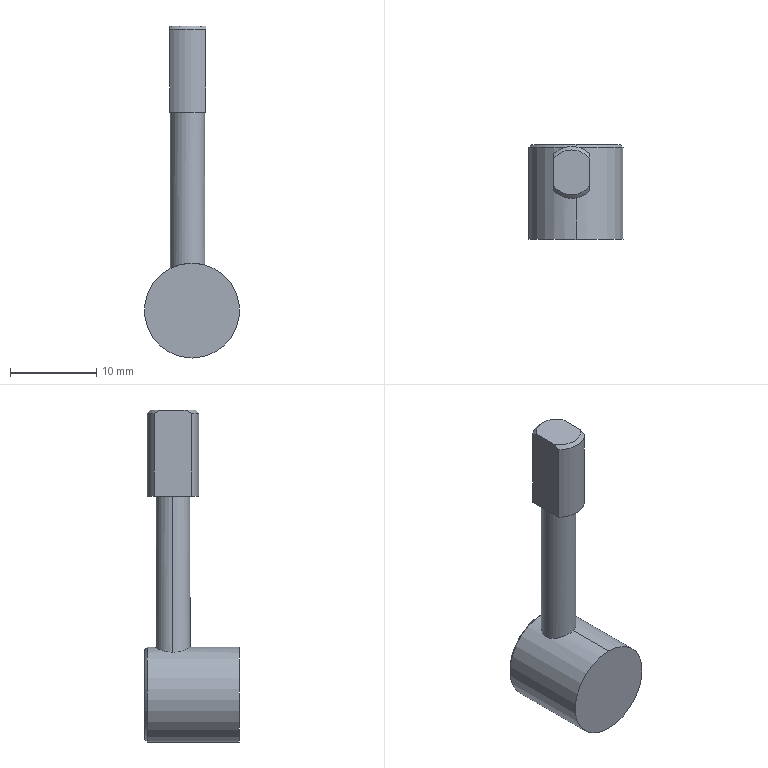Part | STEP file | l_SECWK14 | 1 solid | 23 faces | box 11 x 11 x 38.5 mm | volume 1486 mm3 | cylinder 8 | cone 8 | plane 7 | commonest cylinder face diameters 6 x4 4 x2 11 x2
STEP:
#1=CARTESIAN_POINT('',(-0.5,10.9,-3.));
#2=VERTEX_POINT('',#1);
#3=CARTESIAN_POINT('',(-0.5,10.9,3.));
#4=VERTEX_POINT('',#3);
#5=CARTESIAN_POINT('',(-0.5,10.9,0.));
#6=DIRECTION('',(0.,1.,0.));
#7=DIRECTION('',(0.,0.,1.));
#8=AXIS2_PLACEMENT_3D('',#5,#6,#7);
#9=CIRCLE('',#8,3.);
#10=EDGE_CURVE('',#2,#4,#9,.T.);
#11=ORIENTED_EDGE('',*,*,#10,.T.);
#12=CARTESIAN_POINT('',(-0.5,10.3,3.));
#13=VERTEX_POINT('',#12);
#14=CARTESIAN_POINT('',(-0.5,11.,3.));
#15=DIRECTION('',(0.,-1.,0.));
#16=VECTOR('',#15,1000.);
#17=LINE('',#14,#16);
#18=EDGE_CURVE('',#4,#13,#17,.T.);
#19=ORIENTED_EDGE('',*,*,#18,.T.);
#20=CARTESIAN_POINT('',(-0.5,10.3,-3.));
#21=VERTEX_POINT('',#20);
#22=CARTESIAN_POINT('',(-0.5,10.3,0.));
#23=DIRECTION('',(0.,1.,0.));
#24=DIRECTION('',(0.,0.,-1.));
#25=AXIS2_PLACEMENT_3D('',#22,#23,#24);
#26=CIRCLE('',#25,3.);
#27=EDGE_CURVE('',#21,#13,#26,.T.);
#28=ORIENTED_EDGE('',*,*,#27,.F.);
#29=CARTESIAN_POINT('',(-0.5,11.,-3.));
#30=DIRECTION('',(0.,-1.,0.));
#31=VECTOR('',#30,1000.);
#32=LINE('',#29,#31);
#33=EDGE_CURVE('',#2,#21,#32,.T.);
#34=ORIENTED_EDGE('',*,*,#33,.F.);
#35=EDGE_LOOP('',(#11,#19,#28,#34));
#36=FACE_OUTER_BOUND('',#35,.T.);
#37=CARTESIAN_POINT('',(-0.5,11.,0.));
#38=DIRECTION('',(0.,-1.,0.));
#39=DIRECTION('',(0.,0.,-1.));
#40=AXIS2_PLACEMENT_3D('',#37,#38,#39);
#41=CYLINDRICAL_SURFACE('',#40,3.);
#42=ADVANCED_FACE('',(#36),#41,.F.);
#43=CARTESIAN_POINT('',(-0.5,10.8,2.5));
#44=VERTEX_POINT('',#43);
#45=CARTESIAN_POINT('',(-0.5,10.8,-2.5));
#46=VERTEX_POINT('',#45);
#47=CARTESIAN_POINT('',(-0.5,10.8,0.));
#48=DIRECTION('',(0.,1.,0.));
#49=DIRECTION('',(0.,0.,1.));
#50=AXIS2_PLACEMENT_3D('',#47,#48,#49);
#51=CIRCLE('',#50,2.5);
#52=EDGE_CURVE('',#44,#46,#51,.T.);
#53=ORIENTED_EDGE('',*,*,#52,.F.);
#54=CARTESIAN_POINT('',(-0.5,10.3,3.));
#55=DIRECTION('',(0.,-0.7071,0.7071));
#56=VECTOR('',#55,1000.);
#57=LINE('',#54,#56);
#58=EDGE_CURVE('',#44,#13,#57,.T.);
#59=ORIENTED_EDGE('',*,*,#58,.T.);
#60=CARTESIAN_POINT('',(-0.5,10.3,0.));
#61=DIRECTION('',(0.,1.,0.));
#62=DIRECTION('',(0.,0.,-1.));
#63=AXIS2_PLACEMENT_3D('',#60,#61,#62);
#64=CIRCLE('',#63,3.);
#65=EDGE_CURVE('',#13,#21,#64,.T.);
#66=ORIENTED_EDGE('',*,*,#65,.T.);
#67=CARTESIAN_POINT('',(-0.5,10.3,-3.));
#68=DIRECTION('',(0.,-0.7071,-0.7071));
#69=VECTOR('',#68,1000.);
#70=LINE('',#67,#69);
#71=EDGE_CURVE('',#46,#21,#70,.T.);
#72=ORIENTED_EDGE('',*,*,#71,.F.);
#73=EDGE_LOOP('',(#53,#59,#66,#72));
#74=FACE_OUTER_BOUND('',#73,.T.);
#75=CARTESIAN_POINT('',(-0.5,10.3,0.));
#76=DIRECTION('',(0.,-1.,0.));
#77=DIRECTION('',(0.,0.,-1.));
#78=AXIS2_PLACEMENT_3D('',#75,#76,#77);
#79=CONICAL_SURFACE('',#78,3.,0.7854);
#80=ADVANCED_FACE('',(#74),#79,.T.);
#81=ORIENTED_EDGE('',*,*,#10,.F.);
#82=CARTESIAN_POINT('',(-0.5,11.,-3.1));
#83=VERTEX_POINT('',#82);
#84=CARTESIAN_POINT('',(-0.5,10.9,-3.));
#85=DIRECTION('',(0.,0.7071,-0.7071));
#86=VECTOR('',#85,1000.);
#87=LINE('',#84,#86);
#88=EDGE_CURVE('',#2,#83,#87,.T.);
#89=ORIENTED_EDGE('',*,*,#88,.T.);
#90=CARTESIAN_POINT('',(-0.5,11.,3.1));
#91=VERTEX_POINT('',#90);
#92=CARTESIAN_POINT('',(-0.5,11.,0.));
#93=DIRECTION('',(0.,1.,0.));
#94=DIRECTION('',(0.,0.,1.));
#95=AXIS2_PLACEMENT_3D('',#92,#93,#94);
#96=CIRCLE('',#95,3.1);
#97=EDGE_CURVE('',#83,#91,#96,.T.);
#98=ORIENTED_EDGE('',*,*,#97,.T.);
#99=CARTESIAN_POINT('',(-0.5,10.9,3.));
#100=DIRECTION('',(0.,0.7071,0.7071));
#101=VECTOR('',#100,1000.);
#102=LINE('',#99,#101);
#103=EDGE_CURVE('',#4,#91,#102,.T.);
#104=ORIENTED_EDGE('',*,*,#103,.F.);
#105=EDGE_LOOP('',(#81,#89,#98,#104));
#106=FACE_OUTER_BOUND('',#105,.T.);
#107=CARTESIAN_POINT('',(-0.5,10.9,0.));
#108=DIRECTION('',(0.,1.,0.));
#109=DIRECTION('',(0.,0.,1.));
#110=AXIS2_PLACEMENT_3D('',#107,#108,#109);
#111=CONICAL_SURFACE('',#110,3.,0.7854);
#112=ADVANCED_FACE('',(#106),#111,.F.);
#113=CARTESIAN_POINT('',(0.,11.,5.2));
#114=VERTEX_POINT('',#113);
#115=CARTESIAN_POINT('',(0.,11.,-5.2));
#116=VERTEX_POINT('',#115);
#117=CARTESIAN_POINT('',(0.,11.,0.));
#118=DIRECTION('',(0.,1.,0.));
#119=DIRECTION('',(0.,0.,1.));
#120=AXIS2_PLACEMENT_3D('',#117,#118,#119);
#121=CIRCLE('',#120,5.2);
#122=EDGE_CURVE('',#114,#116,#121,.T.);
#123=ORIENTED_EDGE('',*,*,#122,.F.);
#124=CARTESIAN_POINT('',(0.,10.7,5.5));
#125=VERTEX_POINT('',#124);
#126=CARTESIAN_POINT('',(0.,11.,5.2));
#127=DIRECTION('',(0.,-0.7071,0.7071));
#128=VECTOR('',#127,1000.);
#129=LINE('',#126,#128);
#130=EDGE_CURVE('',#114,#125,#129,.T.);
#131=ORIENTED_EDGE('',*,*,#130,.T.);
#132=CARTESIAN_POINT('',(0.,10.7,-5.5));
#133=VERTEX_POINT('',#132);
#134=CARTESIAN_POINT('',(0.,10.7,0.));
#135=DIRECTION('',(0.,1.,0.));
#136=DIRECTION('',(0.,0.,1.));
#137=AXIS2_PLACEMENT_3D('',#134,#135,#136);
#138=CIRCLE('',#137,5.5);
#139=EDGE_CURVE('',#125,#133,#138,.T.);
#140=ORIENTED_EDGE('',*,*,#139,.T.);
#141=CARTESIAN_POINT('',(0.,11.,-5.2));
#142=DIRECTION('',(0.,-0.7071,-0.7071));
#143=VECTOR('',#142,1000.);
#144=LINE('',#141,#143);
#145=EDGE_CURVE('',#116,#133,#144,.T.);
#146=ORIENTED_EDGE('',*,*,#145,.F.);
#147=EDGE_LOOP('',(#123,#131,#140,#146));
#148=FACE_OUTER_BOUND('',#147,.T.);
#149=CARTESIAN_POINT('',(0.,11.,0.));
#150=DIRECTION('',(0.,-1.,0.));
#151=DIRECTION('',(0.,0.,-1.));
#152=AXIS2_PLACEMENT_3D('',#149,#150,#151);
#153=CONICAL_SURFACE('',#152,5.2,0.7854);
#154=ADVANCED_FACE('',(#148),#153,.T.);
#155=CARTESIAN_POINT('',(-2.5,7.725,4.899));
#156=VERTEX_POINT('',#155);
#157=CARTESIAN_POINT('',(0.,9.661,5.5));
#158=VERTEX_POINT('',#157);
#159=CARTESIAN_POINT('',(-2.5,7.725,4.899));
#160=CARTESIAN_POINT('',(-2.5,7.879,4.899));
#161=CARTESIAN_POINT('',(-2.482,8.034,4.908));
#162=CARTESIAN_POINT('',(-2.411,8.333,4.943));
#163=CARTESIAN_POINT('',(-2.36,8.476,4.969));
#164=CARTESIAN_POINT('',(-2.224,8.75,5.031));
#165=CARTESIAN_POINT('',(-2.142,8.876,5.067));
#166=CARTESIAN_POINT('',(-1.953,9.108,5.143));
#167=CARTESIAN_POINT('',(-1.844,9.213,5.183));
#168=CARTESIAN_POINT('',(-1.491,9.487,5.3));
#169=CARTESIAN_POINT('',(-1.212,9.619,5.373));
#170=CARTESIAN_POINT('',(-0.7662,9.713,5.448));
#171=CARTESIAN_POINT('',(-0.6105,9.728,5.468));
#172=CARTESIAN_POINT('',(-0.304,9.721,5.494));
#173=CARTESIAN_POINT('',(-0.1507,9.7,5.5));
#174=CARTESIAN_POINT('',(0.,9.661,5.5));
#175=B_SPLINE_CURVE_WITH_KNOTS('',3,(#159,#160,#161,#162,#163,#164,#165,#166,#167,#168,#169,#170,#171,#172,#173,#174),.UNSPECIFIED.,.F.,.F.,(4,2,2,2,2,2,2,4),(0.006324,0.006785,0.007246,0.007706,0.008167,0.009089,0.00955,0.01001),.UNSPECIFIED.);
#176=EDGE_CURVE('',#156,#158,#175,.T.);
#177=ORIENTED_EDGE('',*,*,#176,.F.);
#178=CARTESIAN_POINT('',(-2.5,7.725,23.));
#179=VERTEX_POINT('',#178);
#180=CARTESIAN_POINT('',(-2.5,7.725,0.));
#181=DIRECTION('',(0.,0.,1.));
#182=VECTOR('',#181,1000.);
#183=LINE('',#180,#182);
#184=EDGE_CURVE('',#156,#179,#183,.T.);
#185=ORIENTED_EDGE('',*,*,#184,.T.);
#186=CARTESIAN_POINT('',(1.5,7.725,23.));
#187=VERTEX_POINT('',#186);
#188=CARTESIAN_POINT('',(-0.5,7.725,23.));
#189=DIRECTION('',(0.,0.,1.));
#190=DIRECTION('',(1.,0.,0.));
#191=AXIS2_PLACEMENT_3D('',#188,#189,#190);
#192=CIRCLE('',#191,2.);
#193=EDGE_CURVE('',#187,#179,#192,.T.);
#194=ORIENTED_EDGE('',*,*,#193,.F.);
#195=CARTESIAN_POINT('',(1.5,7.725,5.292));
#196=VERTEX_POINT('',#195);
#197=CARTESIAN_POINT('',(1.5,7.725,0.));
#198=DIRECTION('',(0.,0.,1.));
#199=VECTOR('',#198,1000.);
#200=LINE('',#197,#199);
#201=EDGE_CURVE('',#196,#187,#200,.T.);
#202=ORIENTED_EDGE('',*,*,#201,.F.);
#203=CARTESIAN_POINT('',(0.,9.661,5.5));
#204=CARTESIAN_POINT('',(0.2151,9.606,5.5));
#205=CARTESIAN_POINT('',(0.4172,9.516,5.487));
#206=CARTESIAN_POINT('',(0.7858,9.273,5.447));
#207=CARTESIAN_POINT('',(0.9473,9.123,5.42));
#208=CARTESIAN_POINT('',(1.216,8.775,5.366));
#209=CARTESIAN_POINT('',(1.321,8.581,5.34));
#210=CARTESIAN_POINT('',(1.464,8.164,5.302));
#211=CARTESIAN_POINT('',(1.5,7.948,5.292));
#212=CARTESIAN_POINT('',(1.5,7.725,5.292));
#213=B_SPLINE_CURVE_WITH_KNOTS('',3,(#203,#204,#205,#206,#207,#208,#209,#210,#211,#212),.UNSPECIFIED.,.F.,.F.,(4,2,2,2,4),(0.01001,0.01067,0.01133,0.01199,0.01264),.UNSPECIFIED.);
#214=EDGE_CURVE('',#158,#196,#213,.T.);
#215=ORIENTED_EDGE('',*,*,#214,.F.);
#216=EDGE_LOOP('',(#177,#185,#194,#202,#215));
#217=FACE_OUTER_BOUND('',#216,.T.);
#218=CARTESIAN_POINT('',(-0.5,7.725,0.));
#219=DIRECTION('',(0.,0.,1.));
#220=DIRECTION('',(1.,0.,0.));
#221=AXIS2_PLACEMENT_3D('',#218,#219,#220);
#222=CYLINDRICAL_SURFACE('',#221,2.);
#223=ADVANCED_FACE('',(#217),#222,.T.);
#224=ORIENTED_EDGE('',*,*,#139,.F.);
#225=CARTESIAN_POINT('',(0.,11.,5.5));
#226=DIRECTION('',(0.,-1.,0.));
#227=VECTOR('',#226,1000.);
#228=LINE('',#225,#227);
#229=EDGE_CURVE('',#125,#158,#228,.T.);
#230=ORIENTED_EDGE('',*,*,#229,.T.);
#231=ORIENTED_EDGE('',*,*,#214,.T.);
#232=CARTESIAN_POINT('',(0.,5.789,5.5));
#233=VERTEX_POINT('',#232);
#234=CARTESIAN_POINT('',(1.5,7.725,5.292));
#235=CARTESIAN_POINT('',(1.5,7.502,5.292));
#236=CARTESIAN_POINT('',(1.464,7.286,5.302));
#237=CARTESIAN_POINT('',(1.32,6.866,5.34));
#238=CARTESIAN_POINT('',(1.216,6.674,5.366));
#239=CARTESIAN_POINT('',(0.9453,6.325,5.42));
#240=CARTESIAN_POINT('',(0.7855,6.177,5.447));
#241=CARTESIAN_POINT('',(0.4157,5.933,5.487));
#242=CARTESIAN_POINT('',(0.215,5.844,5.5));
#243=CARTESIAN_POINT('',(0.,5.789,5.5));
#244=B_SPLINE_CURVE_WITH_KNOTS('',3,(#234,#235,#236,#237,#238,#239,#240,#241,#242,#243),.UNSPECIFIED.,.F.,.F.,(4,2,2,2,4),(0.,0.0006585,0.001317,0.001975,0.002634),.UNSPECIFIED.);
#245=EDGE_CURVE('',#196,#233,#244,.T.);
#246=ORIENTED_EDGE('',*,*,#245,.T.);
#247=CARTESIAN_POINT('',(0.,0.,5.5));
#248=VERTEX_POINT('',#247);
#249=CARTESIAN_POINT('',(0.,11.,5.5));
#250=DIRECTION('',(0.,-1.,0.));
#251=VECTOR('',#250,1000.);
#252=LINE('',#249,#251);
#253=EDGE_CURVE('',#233,#248,#252,.T.);
#254=ORIENTED_EDGE('',*,*,#253,.T.);
#255=CARTESIAN_POINT('',(0.,0.,-5.5));
#256=VERTEX_POINT('',#255);
#257=CARTESIAN_POINT('',(0.,0.,0.));
#258=DIRECTION('',(0.,1.,0.));
#259=DIRECTION('',(0.,0.,1.));
#260=AXIS2_PLACEMENT_3D('',#257,#258,#259);
#261=CIRCLE('',#260,5.5);
#262=EDGE_CURVE('',#248,#256,#261,.T.);
#263=ORIENTED_EDGE('',*,*,#262,.T.);
#264=CARTESIAN_POINT('',(0.,11.,-5.5));
#265=DIRECTION('',(0.,-1.,0.));
#266=VECTOR('',#265,1000.);
#267=LINE('',#264,#266);
#268=EDGE_CURVE('',#133,#256,#267,.T.);
#269=ORIENTED_EDGE('',*,*,#268,.F.);
#270=EDGE_LOOP('',(#224,#230,#231,#246,#254,#263,#269));
#271=FACE_OUTER_BOUND('',#270,.T.);
#272=CARTESIAN_POINT('',(0.,11.,0.));
#273=DIRECTION('',(0.,-1.,0.));
#274=DIRECTION('',(0.,0.,-1.));
#275=AXIS2_PLACEMENT_3D('',#272,#273,#274);
#276=CYLINDRICAL_SURFACE('',#275,5.5);
#277=ADVANCED_FACE('',(#271),#276,.T.);
#278=CARTESIAN_POINT('',(0.,11.,0.));
#279=DIRECTION('',(0.,1.,0.));
#280=DIRECTION('',(0.,0.,1.));
#281=AXIS2_PLACEMENT_3D('',#278,#279,#280);
#282=CIRCLE('',#281,5.2);
#283=EDGE_CURVE('',#116,#114,#282,.T.);
#284=ORIENTED_EDGE('',*,*,#283,.T.);
#285=ORIENTED_EDGE('',*,*,#122,.T.);
#286=EDGE_LOOP('',(#284,#285));
#287=FACE_OUTER_BOUND('',#286,.T.);
#288=CARTESIAN_POINT('',(-0.5,11.,0.));
#289=DIRECTION('',(0.,1.,0.));
#290=DIRECTION('',(0.,0.,1.));
#291=AXIS2_PLACEMENT_3D('',#288,#289,#290);
#292=CIRCLE('',#291,3.1);
#293=EDGE_CURVE('',#91,#83,#292,.T.);
#294=ORIENTED_EDGE('',*,*,#293,.F.);
#295=ORIENTED_EDGE('',*,*,#97,.F.);
#296=EDGE_LOOP('',(#294,#295));
#297=FACE_BOUND('',#296,.T.);
#298=CARTESIAN_POINT('',(0.,11.,0.));
#299=DIRECTION('',(0.,1.,0.));
#300=DIRECTION('',(0.,0.,1.));
#301=AXIS2_PLACEMENT_3D('',#298,#299,#300);
#302=PLANE('',#301);
#303=ADVANCED_FACE('',(#287,#297),#302,.T.);
#304=ORIENTED_EDGE('',*,*,#229,.F.);
#305=CARTESIAN_POINT('',(0.,10.7,0.));
#306=DIRECTION('',(0.,1.,0.));
#307=DIRECTION('',(0.,0.,1.));
#308=AXIS2_PLACEMENT_3D('',#305,#306,#307);
#309=CIRCLE('',#308,5.5);
#310=EDGE_CURVE('',#133,#125,#309,.T.);
#311=ORIENTED_EDGE('',*,*,#310,.F.);
#312=ORIENTED_EDGE('',*,*,#268,.T.);
#313=CARTESIAN_POINT('',(0.,0.,0.));
#314=DIRECTION('',(0.,1.,0.));
#315=DIRECTION('',(0.,0.,1.));
#316=AXIS2_PLACEMENT_3D('',#313,#314,#315);
#317=CIRCLE('',#316,5.5);
#318=EDGE_CURVE('',#256,#248,#317,.T.);
#319=ORIENTED_EDGE('',*,*,#318,.T.);
#320=ORIENTED_EDGE('',*,*,#253,.F.);
#321=CARTESIAN_POINT('',(0.,5.789,5.5));
#322=CARTESIAN_POINT('',(-0.1506,5.75,5.5));
#323=CARTESIAN_POINT('',(-0.3041,5.729,5.494));
#324=CARTESIAN_POINT('',(-0.6108,5.722,5.468));
#325=CARTESIAN_POINT('',(-0.7665,5.737,5.448));
#326=CARTESIAN_POINT('',(-1.064,5.8,5.398));
#327=CARTESIAN_POINT('',(-1.209,5.849,5.367));
#328=CARTESIAN_POINT('',(-1.483,5.977,5.298));
#329=CARTESIAN_POINT('',(-1.61,6.055,5.261));
#330=CARTESIAN_POINT('',(-1.964,6.33,5.143));
#331=CARTESIAN_POINT('',(-2.158,6.566,5.061));
#332=CARTESIAN_POINT('',(-2.36,6.975,4.968));
#333=CARTESIAN_POINT('',(-2.411,7.117,4.943));
#334=CARTESIAN_POINT('',(-2.482,7.415,4.908));
#335=CARTESIAN_POINT('',(-2.5,7.571,4.899));
#336=CARTESIAN_POINT('',(-2.5,7.725,4.899));
#337=B_SPLINE_CURVE_WITH_KNOTS('',3,(#321,#322,#323,#324,#325,#326,#327,#328,#329,#330,#331,#332,#333,#334,#335,#336),.UNSPECIFIED.,.F.,.F.,(4,2,2,2,2,2,2,4),(0.002634,0.003095,0.003556,0.004018,0.004479,0.005401,0.005862,0.006324),.UNSPECIFIED.);
#338=EDGE_CURVE('',#233,#156,#337,.T.);
#339=ORIENTED_EDGE('',*,*,#338,.T.);
#340=ORIENTED_EDGE('',*,*,#176,.T.);
#341=EDGE_LOOP('',(#304,#311,#312,#319,#320,#339,#340));
#342=FACE_OUTER_BOUND('',#341,.T.);
#343=CARTESIAN_POINT('',(0.,11.,0.));
#344=DIRECTION('',(0.,-1.,0.));
#345=DIRECTION('',(0.,0.,-1.));
#346=AXIS2_PLACEMENT_3D('',#343,#344,#345);
#347=CYLINDRICAL_SURFACE('',#346,5.5);
#348=ADVANCED_FACE('',(#342),#347,.T.);
#349=ORIENTED_EDGE('',*,*,#184,.F.);
#350=ORIENTED_EDGE('',*,*,#338,.F.);
#351=ORIENTED_EDGE('',*,*,#245,.F.);
#352=ORIENTED_EDGE('',*,*,#201,.T.);
#353=CARTESIAN_POINT('',(-0.5,7.725,23.));
#354=DIRECTION('',(0.,0.,1.));
#355=DIRECTION('',(1.,0.,0.));
#356=AXIS2_PLACEMENT_3D('',#353,#354,#355);
#357=CIRCLE('',#356,2.);
#358=EDGE_CURVE('',#179,#187,#357,.T.);
#359=ORIENTED_EDGE('',*,*,#358,.F.);
#360=EDGE_LOOP('',(#349,#350,#351,#352,#359));
#361=FACE_OUTER_BOUND('',#360,.T.);
#362=CARTESIAN_POINT('',(-0.5,7.725,0.));
#363=DIRECTION('',(0.,0.,1.));
#364=DIRECTION('',(1.,0.,0.));
#365=AXIS2_PLACEMENT_3D('',#362,#363,#364);
#366=CYLINDRICAL_SURFACE('',#365,2.);
#367=ADVANCED_FACE('',(#361),#366,.T.);
#368=CARTESIAN_POINT('',(-2.6,9.258,33.));
#369=VERTEX_POINT('',#368);
#370=CARTESIAN_POINT('',(-2.6,6.192,33.));
#371=VERTEX_POINT('',#370);
#372=CARTESIAN_POINT('',(-2.6,16.,33.));
#373=DIRECTION('',(0.,-1.,0.));
#374=VECTOR('',#373,1000.);
#375=LINE('',#372,#374);
#376=EDGE_CURVE('',#369,#371,#375,.T.);
#377=ORIENTED_EDGE('',*,*,#376,.T.);
#378=CARTESIAN_POINT('',(1.6,6.192,33.));
#379=VERTEX_POINT('',#378);
#380=CARTESIAN_POINT('',(-0.5,7.725,33.));
#381=DIRECTION('',(0.,0.,1.));
#382=DIRECTION('',(1.,0.,0.));
#383=AXIS2_PLACEMENT_3D('',#380,#381,#382);
#384=CIRCLE('',#383,2.6);
#385=EDGE_CURVE('',#371,#379,#384,.T.);
#386=ORIENTED_EDGE('',*,*,#385,.T.);
#387=CARTESIAN_POINT('',(1.6,9.258,33.));
#388=VERTEX_POINT('',#387);
#389=CARTESIAN_POINT('',(1.6,0.,33.));
#390=DIRECTION('',(0.,1.,0.));
#391=VECTOR('',#390,1000.);
#392=LINE('',#389,#391);
#393=EDGE_CURVE('',#379,#388,#392,.T.);
#394=ORIENTED_EDGE('',*,*,#393,.T.);
#395=CARTESIAN_POINT('',(-0.5,7.725,33.));
#396=DIRECTION('',(0.,0.,1.));
#397=DIRECTION('',(1.,0.,0.));
#398=AXIS2_PLACEMENT_3D('',#395,#396,#397);
#399=CIRCLE('',#398,2.6);
#400=EDGE_CURVE('',#388,#369,#399,.T.);
#401=ORIENTED_EDGE('',*,*,#400,.T.);
#402=EDGE_LOOP('',(#377,#386,#394,#401));
#403=FACE_OUTER_BOUND('',#402,.T.);
#404=CARTESIAN_POINT('',(-0.5,7.725,33.));
#405=DIRECTION('',(0.,0.,-1.));
#406=DIRECTION('',(-1.,0.,0.));
#407=AXIS2_PLACEMENT_3D('',#404,#405,#406);
#408=PLANE('',#407);
#409=ADVANCED_FACE('',(#403),#408,.F.);
#410=CARTESIAN_POINT('',(-2.6,5.583,32.6));
#411=VERTEX_POINT('',#410);
#412=CARTESIAN_POINT('',(-2.6,5.583,32.6));
#413=CARTESIAN_POINT('',(-2.6,5.78,32.741));
#414=CARTESIAN_POINT('',(-2.6,5.982,32.876));
#415=CARTESIAN_POINT('',(-2.6,6.192,33.));
#416=B_SPLINE_CURVE_WITH_KNOTS('',3,(#412,#413,#414,#415),.UNSPECIFIED.,.F.,.F.,(4,4),(0.005488,0.006221),.UNSPECIFIED.);
#417=EDGE_CURVE('',#411,#371,#416,.T.);
#418=ORIENTED_EDGE('',*,*,#417,.F.);
#419=CARTESIAN_POINT('',(1.6,5.583,32.6));
#420=VERTEX_POINT('',#419);
#421=CARTESIAN_POINT('',(-0.5,7.725,32.6));
#422=DIRECTION('',(0.,0.,1.));
#423=DIRECTION('',(1.,0.,0.));
#424=AXIS2_PLACEMENT_3D('',#421,#422,#423);
#425=CIRCLE('',#424,3.);
#426=EDGE_CURVE('',#411,#420,#425,.T.);
#427=ORIENTED_EDGE('',*,*,#426,.T.);
#428=CARTESIAN_POINT('',(1.6,6.192,33.));
#429=CARTESIAN_POINT('',(1.6,5.983,32.877));
#430=CARTESIAN_POINT('',(1.6,5.781,32.742));
#431=CARTESIAN_POINT('',(1.6,5.583,32.6));
#432=B_SPLINE_CURVE_WITH_KNOTS('',3,(#428,#429,#430,#431),.UNSPECIFIED.,.F.,.F.,(4,4),(0.009429,0.01015),.UNSPECIFIED.);
#433=EDGE_CURVE('',#379,#420,#432,.T.);
#434=ORIENTED_EDGE('',*,*,#433,.F.);
#435=ORIENTED_EDGE('',*,*,#385,.F.);
#436=EDGE_LOOP('',(#418,#427,#434,#435));
#437=FACE_OUTER_BOUND('',#436,.T.);
#438=CARTESIAN_POINT('',(-0.5,7.725,32.6));
#439=DIRECTION('',(0.,0.,-1.));
#440=DIRECTION('',(-1.,0.,0.));
#441=AXIS2_PLACEMENT_3D('',#438,#439,#440);
#442=CONICAL_SURFACE('',#441,3.,0.7854);
#443=ADVANCED_FACE('',(#437),#442,.T.);
#444=CARTESIAN_POINT('',(-2.6,9.867,32.6));
#445=VERTEX_POINT('',#444);
#446=CARTESIAN_POINT('',(-2.6,9.258,33.));
#447=CARTESIAN_POINT('',(-2.6,9.467,32.877));
#448=CARTESIAN_POINT('',(-2.6,9.669,32.742));
#449=CARTESIAN_POINT('',(-2.6,9.867,32.6));
#450=B_SPLINE_CURVE_WITH_KNOTS('',3,(#446,#447,#448,#449),.UNSPECIFIED.,.F.,.F.,(4,4),(0.009429,0.01015),.UNSPECIFIED.);
#451=EDGE_CURVE('',#369,#445,#450,.T.);
#452=ORIENTED_EDGE('',*,*,#451,.F.);
#453=ORIENTED_EDGE('',*,*,#400,.F.);
#454=CARTESIAN_POINT('',(1.6,9.867,32.6));
#455=VERTEX_POINT('',#454);
#456=CARTESIAN_POINT('',(1.6,9.867,32.6));
#457=CARTESIAN_POINT('',(1.6,9.67,32.741));
#458=CARTESIAN_POINT('',(1.6,9.468,32.876));
#459=CARTESIAN_POINT('',(1.6,9.258,33.));
#460=B_SPLINE_CURVE_WITH_KNOTS('',3,(#456,#457,#458,#459),.UNSPECIFIED.,.F.,.F.,(4,4),(0.005488,0.006221),.UNSPECIFIED.);
#461=EDGE_CURVE('',#455,#388,#460,.T.);
#462=ORIENTED_EDGE('',*,*,#461,.F.);
#463=CARTESIAN_POINT('',(-0.5,7.725,32.6));
#464=DIRECTION('',(0.,0.,1.));
#465=DIRECTION('',(1.,0.,0.));
#466=AXIS2_PLACEMENT_3D('',#463,#464,#465);
#467=CIRCLE('',#466,3.);
#468=EDGE_CURVE('',#455,#445,#467,.T.);
#469=ORIENTED_EDGE('',*,*,#468,.T.);
#470=EDGE_LOOP('',(#452,#453,#462,#469));
#471=FACE_OUTER_BOUND('',#470,.T.);
#472=CARTESIAN_POINT('',(-0.5,7.725,32.6));
#473=DIRECTION('',(0.,0.,-1.));
#474=DIRECTION('',(-1.,0.,0.));
#475=AXIS2_PLACEMENT_3D('',#472,#473,#474);
#476=CONICAL_SURFACE('',#475,3.,0.7854);
#477=ADVANCED_FACE('',(#471),#476,.T.);
#478=CARTESIAN_POINT('',(-2.6,5.583,23.));
#479=VERTEX_POINT('',#478);
#480=CARTESIAN_POINT('',(-2.6,5.583,0.));
#481=DIRECTION('',(0.,0.,1.));
#482=VECTOR('',#481,1000.);
#483=LINE('',#480,#482);
#484=EDGE_CURVE('',#479,#411,#483,.T.);
#485=ORIENTED_EDGE('',*,*,#484,.F.);
#486=CARTESIAN_POINT('',(1.6,5.583,23.));
#487=VERTEX_POINT('',#486);
#488=CARTESIAN_POINT('',(-0.5,7.725,23.));
#489=DIRECTION('',(0.,0.,1.));
#490=DIRECTION('',(1.,0.,0.));
#491=AXIS2_PLACEMENT_3D('',#488,#489,#490);
#492=CIRCLE('',#491,3.);
#493=EDGE_CURVE('',#479,#487,#492,.T.);
#494=ORIENTED_EDGE('',*,*,#493,.T.);
#495=CARTESIAN_POINT('',(1.6,5.583,0.));
#496=DIRECTION('',(0.,0.,-1.));
#497=VECTOR('',#496,1000.);
#498=LINE('',#495,#497);
#499=EDGE_CURVE('',#420,#487,#498,.T.);
#500=ORIENTED_EDGE('',*,*,#499,.F.);
#501=ORIENTED_EDGE('',*,*,#426,.F.);
#502=EDGE_LOOP('',(#485,#494,#500,#501));
#503=FACE_OUTER_BOUND('',#502,.T.);
#504=CARTESIAN_POINT('',(-0.5,7.725,0.));
#505=DIRECTION('',(0.,0.,1.));
#506=DIRECTION('',(1.,0.,0.));
#507=AXIS2_PLACEMENT_3D('',#504,#505,#506);
#508=CYLINDRICAL_SURFACE('',#507,3.);
#509=ADVANCED_FACE('',(#503),#508,.T.);
#510=CARTESIAN_POINT('',(-2.6,9.867,23.));
#511=VERTEX_POINT('',#510);
#512=CARTESIAN_POINT('',(-2.6,9.867,0.));
#513=DIRECTION('',(0.,0.,-1.));
#514=VECTOR('',#513,1000.);
#515=LINE('',#512,#514);
#516=EDGE_CURVE('',#445,#511,#515,.T.);
#517=ORIENTED_EDGE('',*,*,#516,.F.);
#518=ORIENTED_EDGE('',*,*,#468,.F.);
#519=CARTESIAN_POINT('',(1.6,9.867,23.));
#520=VERTEX_POINT('',#519);
#521=CARTESIAN_POINT('',(1.6,9.867,0.));
#522=DIRECTION('',(0.,0.,1.));
#523=VECTOR('',#522,1000.);
#524=LINE('',#521,#523);
#525=EDGE_CURVE('',#520,#455,#524,.T.);
#526=ORIENTED_EDGE('',*,*,#525,.F.);
#527=CARTESIAN_POINT('',(-0.5,7.725,23.));
#528=DIRECTION('',(0.,0.,1.));
#529=DIRECTION('',(1.,0.,0.));
#530=AXIS2_PLACEMENT_3D('',#527,#528,#529);
#531=CIRCLE('',#530,3.);
#532=EDGE_CURVE('',#520,#511,#531,.T.);
#533=ORIENTED_EDGE('',*,*,#532,.T.);
#534=EDGE_LOOP('',(#517,#518,#526,#533));
#535=FACE_OUTER_BOUND('',#534,.T.);
#536=CARTESIAN_POINT('',(-0.5,7.725,0.));
#537=DIRECTION('',(0.,0.,1.));
#538=DIRECTION('',(1.,0.,0.));
#539=AXIS2_PLACEMENT_3D('',#536,#537,#538);
#540=CYLINDRICAL_SURFACE('',#539,3.);
#541=ADVANCED_FACE('',(#535),#540,.T.);
#542=ORIENTED_EDGE('',*,*,#193,.T.);
#543=ORIENTED_EDGE('',*,*,#358,.T.);
#544=EDGE_LOOP('',(#542,#543));
#545=FACE_BOUND('',#544,.T.);
#546=CARTESIAN_POINT('',(-2.6,10.725,23.));
#547=DIRECTION('',(0.,-1.,0.));
#548=VECTOR('',#547,1000.);
#549=LINE('',#546,#548);
#550=EDGE_CURVE('',#511,#479,#549,.T.);
#551=ORIENTED_EDGE('',*,*,#550,.F.);
#552=ORIENTED_EDGE('',*,*,#532,.F.);
#553=CARTESIAN_POINT('',(1.6,10.725,23.));
#554=DIRECTION('',(0.,1.,0.));
#555=VECTOR('',#554,1000.);
#556=LINE('',#553,#555);
#557=EDGE_CURVE('',#487,#520,#556,.T.);
#558=ORIENTED_EDGE('',*,*,#557,.F.);
#559=ORIENTED_EDGE('',*,*,#493,.F.);
#560=EDGE_LOOP('',(#551,#552,#558,#559));
#561=FACE_OUTER_BOUND('',#560,.T.);
#562=CARTESIAN_POINT('',(-0.5,10.725,23.));
#563=DIRECTION('',(0.,0.,1.));
#564=DIRECTION('',(1.,0.,0.));
#565=AXIS2_PLACEMENT_3D('',#562,#563,#564);
#566=PLANE('',#565);
#567=ADVANCED_FACE('',(#545,#561),#566,.F.);
#568=ORIENTED_EDGE('',*,*,#461,.T.);
#569=ORIENTED_EDGE('',*,*,#393,.F.);
#570=ORIENTED_EDGE('',*,*,#433,.T.);
#571=ORIENTED_EDGE('',*,*,#499,.T.);
#572=ORIENTED_EDGE('',*,*,#557,.T.);
#573=ORIENTED_EDGE('',*,*,#525,.T.);
#574=EDGE_LOOP('',(#568,#569,#570,#571,#572,#573));
#575=FACE_OUTER_BOUND('',#574,.T.);
#576=CARTESIAN_POINT('',(1.6,0.,23.));
#577=DIRECTION('',(1.,0.,0.));
#578=DIRECTION('',(0.,0.,-1.));
#579=AXIS2_PLACEMENT_3D('',#576,#577,#578);
#580=PLANE('',#579);
#581=ADVANCED_FACE('',(#575),#580,.T.);
#582=ORIENTED_EDGE('',*,*,#417,.T.);
#583=ORIENTED_EDGE('',*,*,#376,.F.);
#584=ORIENTED_EDGE('',*,*,#451,.T.);
#585=ORIENTED_EDGE('',*,*,#516,.T.);
#586=ORIENTED_EDGE('',*,*,#550,.T.);
#587=ORIENTED_EDGE('',*,*,#484,.T.);
#588=EDGE_LOOP('',(#582,#583,#584,#585,#586,#587));
#589=FACE_OUTER_BOUND('',#588,.T.);
#590=CARTESIAN_POINT('',(-2.6,16.,23.));
#591=DIRECTION('',(-1.,0.,0.));
#592=DIRECTION('',(0.,0.,1.));
#593=AXIS2_PLACEMENT_3D('',#590,#591,#592);
#594=PLANE('',#593);
#595=ADVANCED_FACE('',(#589),#594,.T.);
#596=ORIENTED_EDGE('',*,*,#318,.F.);
#597=ORIENTED_EDGE('',*,*,#262,.F.);
#598=EDGE_LOOP('',(#596,#597));
#599=FACE_OUTER_BOUND('',#598,.T.);
#600=CARTESIAN_POINT('',(2.5,0.,0.));
#601=DIRECTION('',(0.,1.,0.));
#602=DIRECTION('',(0.,0.,1.));
#603=AXIS2_PLACEMENT_3D('',#600,#601,#602);
#604=PLANE('',#603);
#605=ADVANCED_FACE('',(#599),#604,.F.);
#606=ORIENTED_EDGE('',*,*,#130,.F.);
#607=ORIENTED_EDGE('',*,*,#283,.F.);
#608=ORIENTED_EDGE('',*,*,#145,.T.);
#609=ORIENTED_EDGE('',*,*,#310,.T.);
#610=EDGE_LOOP('',(#606,#607,#608,#609));
#611=FACE_OUTER_BOUND('',#610,.T.);
#612=CARTESIAN_POINT('',(0.,11.,0.));
#613=DIRECTION('',(0.,-1.,0.));
#614=DIRECTION('',(0.,0.,-1.));
#615=AXIS2_PLACEMENT_3D('',#612,#613,#614);
#616=CONICAL_SURFACE('',#615,5.2,0.7854);
#617=ADVANCED_FACE('',(#611),#616,.T.);
#618=ORIENTED_EDGE('',*,*,#88,.F.);
#619=CARTESIAN_POINT('',(-0.5,10.9,0.));
#620=DIRECTION('',(0.,1.,0.));
#621=DIRECTION('',(0.,0.,1.));
#622=AXIS2_PLACEMENT_3D('',#619,#620,#621);
#623=CIRCLE('',#622,3.);
#624=EDGE_CURVE('',#4,#2,#623,.T.);
#625=ORIENTED_EDGE('',*,*,#624,.F.);
#626=ORIENTED_EDGE('',*,*,#103,.T.);
#627=ORIENTED_EDGE('',*,*,#293,.T.);
#628=EDGE_LOOP('',(#618,#625,#626,#627));
#629=FACE_OUTER_BOUND('',#628,.T.);
#630=CARTESIAN_POINT('',(-0.5,10.9,0.));
#631=DIRECTION('',(0.,1.,0.));
#632=DIRECTION('',(0.,0.,1.));
#633=AXIS2_PLACEMENT_3D('',#630,#631,#632);
#634=CONICAL_SURFACE('',#633,3.,0.7854);
#635=ADVANCED_FACE('',(#629),#634,.F.);
#636=CARTESIAN_POINT('',(-0.5,10.8,0.));
#637=DIRECTION('',(0.,1.,0.));
#638=DIRECTION('',(0.,0.,1.));
#639=AXIS2_PLACEMENT_3D('',#636,#637,#638);
#640=CIRCLE('',#639,2.5);
#641=EDGE_CURVE('',#46,#44,#640,.T.);
#642=ORIENTED_EDGE('',*,*,#641,.T.);
#643=ORIENTED_EDGE('',*,*,#52,.T.);
#644=EDGE_LOOP('',(#642,#643));
#645=FACE_OUTER_BOUND('',#644,.T.);
#646=CARTESIAN_POINT('',(-0.5,10.8,0.));
#647=DIRECTION('',(0.,-1.,0.));
#648=DIRECTION('',(0.,0.,-1.));
#649=AXIS2_PLACEMENT_3D('',#646,#647,#648);
#650=PLANE('',#649);
#651=ADVANCED_FACE('',(#645),#650,.F.);
#652=ORIENTED_EDGE('',*,*,#58,.F.);
#653=ORIENTED_EDGE('',*,*,#641,.F.);
#654=ORIENTED_EDGE('',*,*,#71,.T.);
#655=ORIENTED_EDGE('',*,*,#27,.T.);
#656=EDGE_LOOP('',(#652,#653,#654,#655));
#657=FACE_OUTER_BOUND('',#656,.T.);
#658=CARTESIAN_POINT('',(-0.5,10.3,0.));
#659=DIRECTION('',(0.,-1.,0.));
#660=DIRECTION('',(0.,0.,-1.));
#661=AXIS2_PLACEMENT_3D('',#658,#659,#660);
#662=CONICAL_SURFACE('',#661,3.,0.7854);
#663=ADVANCED_FACE('',(#657),#662,.T.);
#664=ORIENTED_EDGE('',*,*,#18,.F.);
#665=ORIENTED_EDGE('',*,*,#624,.T.);
#666=ORIENTED_EDGE('',*,*,#33,.T.);
#667=ORIENTED_EDGE('',*,*,#65,.F.);
#668=EDGE_LOOP('',(#664,#665,#666,#667));
#669=FACE_OUTER_BOUND('',#668,.T.);
#670=CARTESIAN_POINT('',(-0.5,11.,0.));
#671=DIRECTION('',(0.,-1.,0.));
#672=DIRECTION('',(0.,0.,-1.));
#673=AXIS2_PLACEMENT_3D('',#670,#671,#672);
#674=CYLINDRICAL_SURFACE('',#673,3.);
#675=ADVANCED_FACE('',(#669),#674,.F.);
#676=CLOSED_SHELL('',(#42,#80,#112,#154,#223,#277,#303,#348,#367,#409,#443,#477,#509,#541,#567,#581,#595,#605,#617,#635,#651,#663,#675));
#677=MANIFOLD_SOLID_BREP('',#676);
#678=CARTESIAN_POINT('',(0.,0.,0.));
#679=DIRECTION('',(0.,0.,1.));
#680=DIRECTION('',(1.,0.,0.));
#681=AXIS2_PLACEMENT_3D('',#678,#679,#680);
#682=(LENGTH_UNIT()NAMED_UNIT(*)SI_UNIT(.MILLI.,.METRE.));
#683=UNCERTAINTY_MEASURE_WITH_UNIT(LENGTH_MEASURE(0.00001),#682,'','');
#684=(NAMED_UNIT(*)PLANE_ANGLE_UNIT()SI_UNIT($,.RADIAN.));
#685=(NAMED_UNIT(*)SI_UNIT($,.STERADIAN.)SOLID_ANGLE_UNIT());
#686=(GEOMETRIC_REPRESENTATION_CONTEXT(3)GLOBAL_UNCERTAINTY_ASSIGNED_CONTEXT((#683))GLOBAL_UNIT_ASSIGNED_CONTEXT((#682,#684,#685))REPRESENTATION_CONTEXT('',''));
#687=ADVANCED_BREP_SHAPE_REPRESENTATION('',(#677,#681),#686);